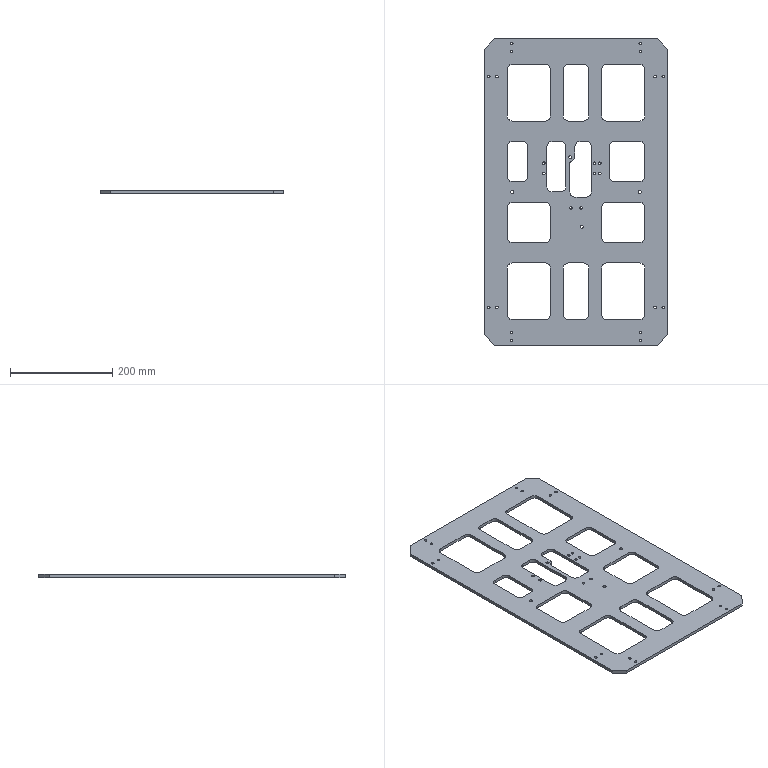Part | SolidWorks | features Extrusion 1 | 1 solid | 165 faces | box 360 x 600 x 6 mm | volume 820919 mm3 | cylinder 106 | plane 59 | commonest cylinder face diameters 20 x49 5 x48 6 x8 10 x1